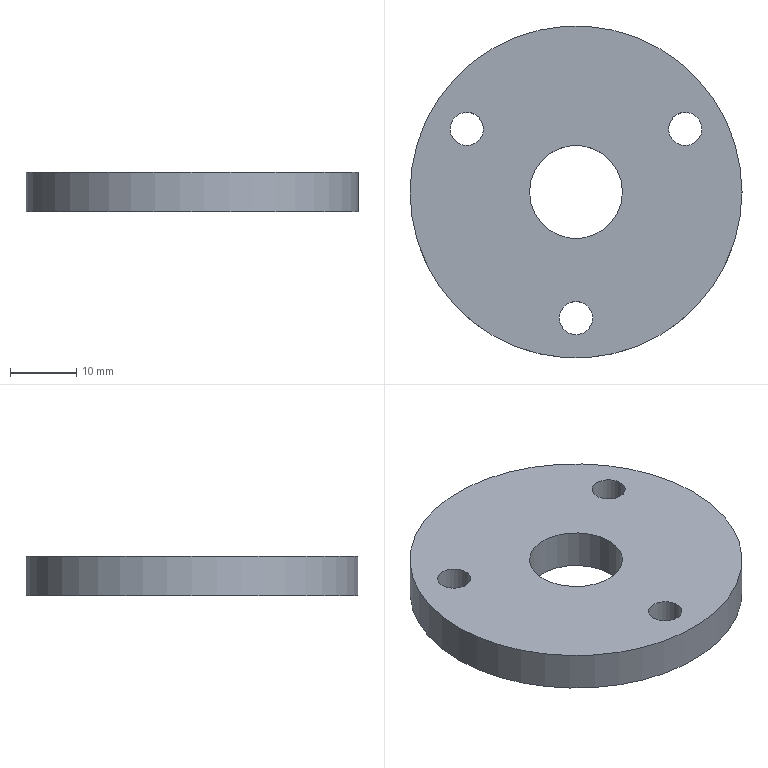Part | NX | features DATUM_CSYS 2, EXTRUDE 1, SKETCH 1 | 1 solid | 7 faces | box 50 x 50 x 6 mm | volume 10504 mm3 | cylinder 5 | plane 2 | commonest cylinder face diameters 5 x3 14 x1 50 x1
STEP:
#1=CARTESIAN_POINT('',(7.,0.,3.));
#2=VERTEX_POINT('',#1);
#3=CARTESIAN_POINT('',(0.,0.,3.));
#4=DIRECTION('',(0.,0.,1.));
#5=DIRECTION('',(1.,0.,0.));
#6=AXIS2_PLACEMENT_3D('',#3,#4,#5);
#7=CIRCLE('',#6,7.);
#8=EDGE_CURVE('',#2,#2,#7,.T.);
#9=ORIENTED_EDGE('',*,*,#8,.T.);
#10=EDGE_LOOP('',(#9));
#11=FACE_BOUND('',#10,.T.);
#12=CARTESIAN_POINT('',(7.,0.,-3.));
#13=VERTEX_POINT('',#12);
#14=CARTESIAN_POINT('',(0.,0.,-3.));
#15=DIRECTION('',(0.,0.,1.));
#16=DIRECTION('',(1.,0.,0.));
#17=AXIS2_PLACEMENT_3D('',#14,#15,#16);
#18=CIRCLE('',#17,7.);
#19=EDGE_CURVE('',#13,#13,#18,.T.);
#20=ORIENTED_EDGE('',*,*,#19,.F.);
#21=EDGE_LOOP('',(#20));
#22=FACE_BOUND('',#21,.T.);
#23=CARTESIAN_POINT('',(0.,0.,3.));
#24=DIRECTION('',(0.,0.,-1.));
#25=DIRECTION('',(-1.,0.,0.));
#26=AXIS2_PLACEMENT_3D('',#23,#24,#25);
#27=CYLINDRICAL_SURFACE('',#26,7.);
#28=ADVANCED_FACE('',(#11,#22),#27,.F.);
#29=CARTESIAN_POINT('',(2.5,-19.,3.));
#30=VERTEX_POINT('',#29);
#31=CARTESIAN_POINT('',(0.,-19.,3.));
#32=DIRECTION('',(0.,0.,1.));
#33=DIRECTION('',(1.,0.,0.));
#34=AXIS2_PLACEMENT_3D('',#31,#32,#33);
#35=CIRCLE('',#34,2.5);
#36=EDGE_CURVE('',#30,#30,#35,.T.);
#37=ORIENTED_EDGE('',*,*,#36,.T.);
#38=EDGE_LOOP('',(#37));
#39=FACE_BOUND('',#38,.T.);
#40=CARTESIAN_POINT('',(2.5,-19.,-3.));
#41=VERTEX_POINT('',#40);
#42=CARTESIAN_POINT('',(0.,-19.,-3.));
#43=DIRECTION('',(0.,0.,1.));
#44=DIRECTION('',(1.,0.,0.));
#45=AXIS2_PLACEMENT_3D('',#42,#43,#44);
#46=CIRCLE('',#45,2.5);
#47=EDGE_CURVE('',#41,#41,#46,.T.);
#48=ORIENTED_EDGE('',*,*,#47,.F.);
#49=EDGE_LOOP('',(#48));
#50=FACE_BOUND('',#49,.T.);
#51=CARTESIAN_POINT('',(0.,-19.,3.));
#52=DIRECTION('',(0.,0.,-1.));
#53=DIRECTION('',(-1.,0.,0.));
#54=AXIS2_PLACEMENT_3D('',#51,#52,#53);
#55=CYLINDRICAL_SURFACE('',#54,2.5);
#56=ADVANCED_FACE('',(#39,#50),#55,.F.);
#57=CARTESIAN_POINT('',(15.204,11.665,3.));
#58=VERTEX_POINT('',#57);
#59=CARTESIAN_POINT('',(16.454,9.5,3.));
#60=DIRECTION('',(0.,0.,1.));
#61=DIRECTION('',(-0.5,0.866,0.));
#62=AXIS2_PLACEMENT_3D('',#59,#60,#61);
#63=CIRCLE('',#62,2.5);
#64=EDGE_CURVE('',#58,#58,#63,.T.);
#65=ORIENTED_EDGE('',*,*,#64,.T.);
#66=EDGE_LOOP('',(#65));
#67=FACE_BOUND('',#66,.T.);
#68=CARTESIAN_POINT('',(15.204,11.665,-3.));
#69=VERTEX_POINT('',#68);
#70=CARTESIAN_POINT('',(16.454,9.5,-3.));
#71=DIRECTION('',(0.,0.,1.));
#72=DIRECTION('',(-0.5,0.866,0.));
#73=AXIS2_PLACEMENT_3D('',#70,#71,#72);
#74=CIRCLE('',#73,2.5);
#75=EDGE_CURVE('',#69,#69,#74,.T.);
#76=ORIENTED_EDGE('',*,*,#75,.F.);
#77=EDGE_LOOP('',(#76));
#78=FACE_BOUND('',#77,.T.);
#79=CARTESIAN_POINT('',(16.454,9.5,3.));
#80=DIRECTION('',(0.,0.,-1.));
#81=DIRECTION('',(-1.,0.,0.));
#82=AXIS2_PLACEMENT_3D('',#79,#80,#81);
#83=CYLINDRICAL_SURFACE('',#82,2.5);
#84=ADVANCED_FACE('',(#67,#78),#83,.F.);
#85=CARTESIAN_POINT('',(25.,0.,3.));
#86=VERTEX_POINT('',#85);
#87=CARTESIAN_POINT('',(0.,0.,3.));
#88=DIRECTION('',(0.,0.,1.));
#89=DIRECTION('',(1.,0.,0.));
#90=AXIS2_PLACEMENT_3D('',#87,#88,#89);
#91=CIRCLE('',#90,25.);
#92=EDGE_CURVE('',#86,#86,#91,.T.);
#93=ORIENTED_EDGE('',*,*,#92,.F.);
#94=EDGE_LOOP('',(#93));
#95=FACE_BOUND('',#94,.T.);
#96=CARTESIAN_POINT('',(25.,0.,-3.));
#97=VERTEX_POINT('',#96);
#98=CARTESIAN_POINT('',(0.,0.,-3.));
#99=DIRECTION('',(0.,0.,1.));
#100=DIRECTION('',(1.,0.,0.));
#101=AXIS2_PLACEMENT_3D('',#98,#99,#100);
#102=CIRCLE('',#101,25.);
#103=EDGE_CURVE('',#97,#97,#102,.T.);
#104=ORIENTED_EDGE('',*,*,#103,.T.);
#105=EDGE_LOOP('',(#104));
#106=FACE_BOUND('',#105,.T.);
#107=CARTESIAN_POINT('',(0.,0.,3.));
#108=DIRECTION('',(0.,0.,-1.));
#109=DIRECTION('',(-1.,0.,0.));
#110=AXIS2_PLACEMENT_3D('',#107,#108,#109);
#111=CYLINDRICAL_SURFACE('',#110,25.);
#112=ADVANCED_FACE('',(#95,#106),#111,.T.);
#113=CARTESIAN_POINT('',(-17.704,7.335,3.));
#114=VERTEX_POINT('',#113);
#115=CARTESIAN_POINT('',(-16.454,9.5,3.));
#116=DIRECTION('',(0.,0.,1.));
#117=DIRECTION('',(-0.5,-0.866,0.));
#118=AXIS2_PLACEMENT_3D('',#115,#116,#117);
#119=CIRCLE('',#118,2.5);
#120=EDGE_CURVE('',#114,#114,#119,.T.);
#121=ORIENTED_EDGE('',*,*,#120,.T.);
#122=EDGE_LOOP('',(#121));
#123=FACE_BOUND('',#122,.T.);
#124=CARTESIAN_POINT('',(-17.704,7.335,-3.));
#125=VERTEX_POINT('',#124);
#126=CARTESIAN_POINT('',(-16.454,9.5,-3.));
#127=DIRECTION('',(0.,0.,1.));
#128=DIRECTION('',(-0.5,-0.866,0.));
#129=AXIS2_PLACEMENT_3D('',#126,#127,#128);
#130=CIRCLE('',#129,2.5);
#131=EDGE_CURVE('',#125,#125,#130,.T.);
#132=ORIENTED_EDGE('',*,*,#131,.F.);
#133=EDGE_LOOP('',(#132));
#134=FACE_BOUND('',#133,.T.);
#135=CARTESIAN_POINT('',(-16.454,9.5,3.));
#136=DIRECTION('',(0.,0.,-1.));
#137=DIRECTION('',(-1.,0.,0.));
#138=AXIS2_PLACEMENT_3D('',#135,#136,#137);
#139=CYLINDRICAL_SURFACE('',#138,2.5);
#140=ADVANCED_FACE('',(#123,#134),#139,.F.);
#141=ORIENTED_EDGE('',*,*,#92,.T.);
#142=EDGE_LOOP('',(#141));
#143=FACE_BOUND('',#142,.T.);
#144=ORIENTED_EDGE('',*,*,#64,.F.);
#145=EDGE_LOOP('',(#144));
#146=FACE_BOUND('',#145,.T.);
#147=ORIENTED_EDGE('',*,*,#36,.F.);
#148=EDGE_LOOP('',(#147));
#149=FACE_BOUND('',#148,.T.);
#150=ORIENTED_EDGE('',*,*,#8,.F.);
#151=EDGE_LOOP('',(#150));
#152=FACE_BOUND('',#151,.T.);
#153=ORIENTED_EDGE('',*,*,#120,.F.);
#154=EDGE_LOOP('',(#153));
#155=FACE_BOUND('',#154,.T.);
#156=CARTESIAN_POINT('',(8.227,4.75,3.));
#157=DIRECTION('',(0.,0.,1.));
#158=DIRECTION('',(1.,0.,0.));
#159=AXIS2_PLACEMENT_3D('',#156,#157,#158);
#160=PLANE('',#159);
#161=ADVANCED_FACE('',(#143,#146,#149,#152,#155),#160,.T.);
#162=ORIENTED_EDGE('',*,*,#103,.F.);
#163=EDGE_LOOP('',(#162));
#164=FACE_BOUND('',#163,.T.);
#165=ORIENTED_EDGE('',*,*,#75,.T.);
#166=EDGE_LOOP('',(#165));
#167=FACE_BOUND('',#166,.T.);
#168=ORIENTED_EDGE('',*,*,#47,.T.);
#169=EDGE_LOOP('',(#168));
#170=FACE_BOUND('',#169,.T.);
#171=ORIENTED_EDGE('',*,*,#19,.T.);
#172=EDGE_LOOP('',(#171));
#173=FACE_BOUND('',#172,.T.);
#174=ORIENTED_EDGE('',*,*,#131,.T.);
#175=EDGE_LOOP('',(#174));
#176=FACE_BOUND('',#175,.T.);
#177=CARTESIAN_POINT('',(8.227,4.75,-3.));
#178=DIRECTION('',(0.,0.,1.));
#179=DIRECTION('',(1.,0.,0.));
#180=AXIS2_PLACEMENT_3D('',#177,#178,#179);
#181=PLANE('',#180);
#182=ADVANCED_FACE('',(#164,#167,#170,#173,#176),#181,.F.);
#183=CLOSED_SHELL('',(#28,#56,#84,#112,#140,#161,#182));
#184=MANIFOLD_SOLID_BREP('',#183);
#185=(LENGTH_UNIT()NAMED_UNIT(*)SI_UNIT(.MILLI.,.METRE.));
#186=UNCERTAINTY_MEASURE_WITH_UNIT(LENGTH_MEASURE(0.00001),#185,'','');
#187=(NAMED_UNIT(*)PLANE_ANGLE_UNIT()SI_UNIT($,.RADIAN.));
#188=(NAMED_UNIT(*)SI_UNIT($,.STERADIAN.)SOLID_ANGLE_UNIT());
#189=(GEOMETRIC_REPRESENTATION_CONTEXT(3)GLOBAL_UNCERTAINTY_ASSIGNED_CONTEXT((#186))GLOBAL_UNIT_ASSIGNED_CONTEXT((#185,#187,#188))REPRESENTATION_CONTEXT('',''));
#190=ADVANCED_BREP_SHAPE_REPRESENTATION('',(#184),#189);